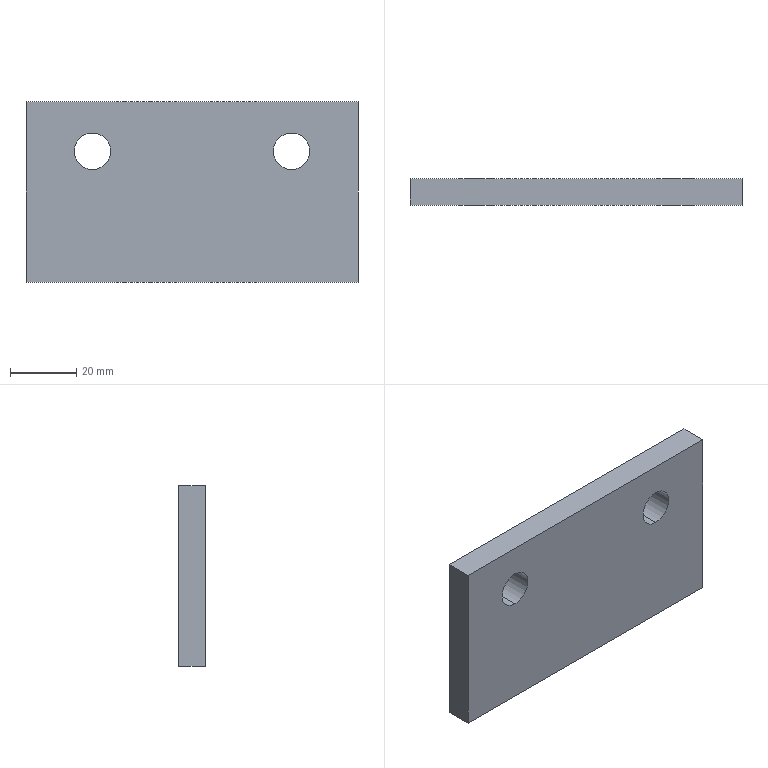Part | SolidWorks | features Extrusion 1, HoleWzd 1 | 1 solid | 10 faces | box 100 x 8 x 54.5 mm | volume 42079 mm3 | plane 6 | cylinder 4 | commonest cylinder face diameters 11 x4
STEP:
#1=CARTESIAN_POINT('',(-30.,0.,6.75));
#2=VERTEX_POINT('',#1);
#3=CARTESIAN_POINT('',(-30.,0.,17.75));
#4=VERTEX_POINT('',#3);
#5=CARTESIAN_POINT('',(-30.,0.,12.25));
#6=DIRECTION('',(0.,1.,0.));
#7=DIRECTION('',(0.,0.,1.));
#8=AXIS2_PLACEMENT_3D('',#5,#6,#7);
#9=CIRCLE('',#8,5.5);
#10=EDGE_CURVE('',#2,#4,#9,.T.);
#11=ORIENTED_EDGE('',*,*,#10,.F.);
#12=CARTESIAN_POINT('',(-30.,8.,6.75));
#13=VERTEX_POINT('',#12);
#14=CARTESIAN_POINT('',(-30.,8.,6.75));
#15=DIRECTION('',(0.,1.,0.));
#16=VECTOR('',#15,1000.);
#17=LINE('',#14,#16);
#18=EDGE_CURVE('',#2,#13,#17,.T.);
#19=ORIENTED_EDGE('',*,*,#18,.T.);
#20=CARTESIAN_POINT('',(-30.,8.,17.75));
#21=VERTEX_POINT('',#20);
#22=CARTESIAN_POINT('',(-30.,8.,12.25));
#23=DIRECTION('',(0.,1.,0.));
#24=DIRECTION('',(0.,0.,1.));
#25=AXIS2_PLACEMENT_3D('',#22,#23,#24);
#26=CIRCLE('',#25,5.5);
#27=EDGE_CURVE('',#13,#21,#26,.T.);
#28=ORIENTED_EDGE('',*,*,#27,.T.);
#29=CARTESIAN_POINT('',(-30.,8.,17.75));
#30=DIRECTION('',(0.,1.,0.));
#31=VECTOR('',#30,1000.);
#32=LINE('',#29,#31);
#33=EDGE_CURVE('',#4,#21,#32,.T.);
#34=ORIENTED_EDGE('',*,*,#33,.F.);
#35=EDGE_LOOP('',(#11,#19,#28,#34));
#36=FACE_OUTER_BOUND('',#35,.T.);
#37=CARTESIAN_POINT('',(-30.,8.,12.25));
#38=DIRECTION('',(0.,1.,0.));
#39=DIRECTION('',(0.,0.,1.));
#40=AXIS2_PLACEMENT_3D('',#37,#38,#39);
#41=CYLINDRICAL_SURFACE('',#40,5.5);
#42=ADVANCED_FACE('',(#36),#41,.F.);
#43=CARTESIAN_POINT('',(30.,0.,6.75));
#44=VERTEX_POINT('',#43);
#45=CARTESIAN_POINT('',(30.,0.,17.75));
#46=VERTEX_POINT('',#45);
#47=CARTESIAN_POINT('',(30.,0.,12.25));
#48=DIRECTION('',(0.,1.,0.));
#49=DIRECTION('',(0.,0.,1.));
#50=AXIS2_PLACEMENT_3D('',#47,#48,#49);
#51=CIRCLE('',#50,5.5);
#52=EDGE_CURVE('',#44,#46,#51,.T.);
#53=ORIENTED_EDGE('',*,*,#52,.F.);
#54=CARTESIAN_POINT('',(30.,8.,6.75));
#55=VERTEX_POINT('',#54);
#56=CARTESIAN_POINT('',(30.,8.,6.75));
#57=DIRECTION('',(0.,1.,0.));
#58=VECTOR('',#57,1000.);
#59=LINE('',#56,#58);
#60=EDGE_CURVE('',#44,#55,#59,.T.);
#61=ORIENTED_EDGE('',*,*,#60,.T.);
#62=CARTESIAN_POINT('',(30.,8.,17.75));
#63=VERTEX_POINT('',#62);
#64=CARTESIAN_POINT('',(30.,8.,12.25));
#65=DIRECTION('',(0.,1.,0.));
#66=DIRECTION('',(0.,0.,1.));
#67=AXIS2_PLACEMENT_3D('',#64,#65,#66);
#68=CIRCLE('',#67,5.5);
#69=EDGE_CURVE('',#55,#63,#68,.T.);
#70=ORIENTED_EDGE('',*,*,#69,.T.);
#71=CARTESIAN_POINT('',(30.,8.,17.75));
#72=DIRECTION('',(0.,1.,0.));
#73=VECTOR('',#72,1000.);
#74=LINE('',#71,#73);
#75=EDGE_CURVE('',#46,#63,#74,.T.);
#76=ORIENTED_EDGE('',*,*,#75,.F.);
#77=EDGE_LOOP('',(#53,#61,#70,#76));
#78=FACE_OUTER_BOUND('',#77,.T.);
#79=CARTESIAN_POINT('',(30.,8.,12.25));
#80=DIRECTION('',(0.,1.,0.));
#81=DIRECTION('',(0.,0.,1.));
#82=AXIS2_PLACEMENT_3D('',#79,#80,#81);
#83=CYLINDRICAL_SURFACE('',#82,5.5);
#84=ADVANCED_FACE('',(#78),#83,.F.);
#85=CARTESIAN_POINT('',(-50.,0.,-27.25));
#86=VERTEX_POINT('',#85);
#87=CARTESIAN_POINT('',(-50.,0.,27.25));
#88=VERTEX_POINT('',#87);
#89=CARTESIAN_POINT('',(-50.,0.,27.25));
#90=DIRECTION('',(0.,0.,1.));
#91=VECTOR('',#90,1000.);
#92=LINE('',#89,#91);
#93=EDGE_CURVE('',#86,#88,#92,.T.);
#94=ORIENTED_EDGE('',*,*,#93,.T.);
#95=CARTESIAN_POINT('',(-50.,8.,27.25));
#96=VERTEX_POINT('',#95);
#97=CARTESIAN_POINT('',(-50.,8.,27.25));
#98=DIRECTION('',(0.,-1.,0.));
#99=VECTOR('',#98,1000.);
#100=LINE('',#97,#99);
#101=EDGE_CURVE('',#96,#88,#100,.T.);
#102=ORIENTED_EDGE('',*,*,#101,.F.);
#103=CARTESIAN_POINT('',(-50.,8.,-27.25));
#104=VERTEX_POINT('',#103);
#105=CARTESIAN_POINT('',(-50.,8.,27.25));
#106=DIRECTION('',(0.,0.,1.));
#107=VECTOR('',#106,1000.);
#108=LINE('',#105,#107);
#109=EDGE_CURVE('',#104,#96,#108,.T.);
#110=ORIENTED_EDGE('',*,*,#109,.F.);
#111=CARTESIAN_POINT('',(-50.,8.,-27.25));
#112=DIRECTION('',(0.,-1.,0.));
#113=VECTOR('',#112,1000.);
#114=LINE('',#111,#113);
#115=EDGE_CURVE('',#104,#86,#114,.T.);
#116=ORIENTED_EDGE('',*,*,#115,.T.);
#117=EDGE_LOOP('',(#94,#102,#110,#116));
#118=FACE_OUTER_BOUND('',#117,.T.);
#119=CARTESIAN_POINT('',(-50.,8.,27.25));
#120=DIRECTION('',(1.,0.,0.));
#121=DIRECTION('',(0.,0.,-1.));
#122=AXIS2_PLACEMENT_3D('',#119,#120,#121);
#123=PLANE('',#122);
#124=ADVANCED_FACE('',(#118),#123,.F.);
#125=CARTESIAN_POINT('',(50.,0.,27.25));
#126=VERTEX_POINT('',#125);
#127=CARTESIAN_POINT('',(50.,0.,27.25));
#128=DIRECTION('',(1.,0.,0.));
#129=VECTOR('',#128,1000.);
#130=LINE('',#127,#129);
#131=EDGE_CURVE('',#88,#126,#130,.T.);
#132=ORIENTED_EDGE('',*,*,#131,.T.);
#133=CARTESIAN_POINT('',(50.,8.,27.25));
#134=VERTEX_POINT('',#133);
#135=CARTESIAN_POINT('',(50.,8.,27.25));
#136=DIRECTION('',(0.,-1.,0.));
#137=VECTOR('',#136,1000.);
#138=LINE('',#135,#137);
#139=EDGE_CURVE('',#134,#126,#138,.T.);
#140=ORIENTED_EDGE('',*,*,#139,.F.);
#141=CARTESIAN_POINT('',(50.,8.,27.25));
#142=DIRECTION('',(1.,0.,0.));
#143=VECTOR('',#142,1000.);
#144=LINE('',#141,#143);
#145=EDGE_CURVE('',#96,#134,#144,.T.);
#146=ORIENTED_EDGE('',*,*,#145,.F.);
#147=ORIENTED_EDGE('',*,*,#101,.T.);
#148=EDGE_LOOP('',(#132,#140,#146,#147));
#149=FACE_OUTER_BOUND('',#148,.T.);
#150=CARTESIAN_POINT('',(50.,8.,27.25));
#151=DIRECTION('',(0.,0.,-1.));
#152=DIRECTION('',(-1.,0.,0.));
#153=AXIS2_PLACEMENT_3D('',#150,#151,#152);
#154=PLANE('',#153);
#155=ADVANCED_FACE('',(#149),#154,.F.);
#156=CARTESIAN_POINT('',(50.,0.,-27.25));
#157=VERTEX_POINT('',#156);
#158=CARTESIAN_POINT('',(50.,0.,27.25));
#159=DIRECTION('',(0.,0.,-1.));
#160=VECTOR('',#159,1000.);
#161=LINE('',#158,#160);
#162=EDGE_CURVE('',#126,#157,#161,.T.);
#163=ORIENTED_EDGE('',*,*,#162,.T.);
#164=CARTESIAN_POINT('',(50.,8.,-27.25));
#165=VERTEX_POINT('',#164);
#166=CARTESIAN_POINT('',(50.,8.,-27.25));
#167=DIRECTION('',(0.,-1.,0.));
#168=VECTOR('',#167,1000.);
#169=LINE('',#166,#168);
#170=EDGE_CURVE('',#165,#157,#169,.T.);
#171=ORIENTED_EDGE('',*,*,#170,.F.);
#172=CARTESIAN_POINT('',(50.,8.,27.25));
#173=DIRECTION('',(0.,0.,-1.));
#174=VECTOR('',#173,1000.);
#175=LINE('',#172,#174);
#176=EDGE_CURVE('',#134,#165,#175,.T.);
#177=ORIENTED_EDGE('',*,*,#176,.F.);
#178=ORIENTED_EDGE('',*,*,#139,.T.);
#179=EDGE_LOOP('',(#163,#171,#177,#178));
#180=FACE_OUTER_BOUND('',#179,.T.);
#181=CARTESIAN_POINT('',(50.,8.,27.25));
#182=DIRECTION('',(-1.,0.,0.));
#183=DIRECTION('',(0.,0.,1.));
#184=AXIS2_PLACEMENT_3D('',#181,#182,#183);
#185=PLANE('',#184);
#186=ADVANCED_FACE('',(#180),#185,.F.);
#187=CARTESIAN_POINT('',(50.,0.,-27.25));
#188=DIRECTION('',(-1.,0.,0.));
#189=VECTOR('',#188,1000.);
#190=LINE('',#187,#189);
#191=EDGE_CURVE('',#157,#86,#190,.T.);
#192=ORIENTED_EDGE('',*,*,#191,.T.);
#193=ORIENTED_EDGE('',*,*,#115,.F.);
#194=CARTESIAN_POINT('',(50.,8.,-27.25));
#195=DIRECTION('',(-1.,0.,0.));
#196=VECTOR('',#195,1000.);
#197=LINE('',#194,#196);
#198=EDGE_CURVE('',#165,#104,#197,.T.);
#199=ORIENTED_EDGE('',*,*,#198,.F.);
#200=ORIENTED_EDGE('',*,*,#170,.T.);
#201=EDGE_LOOP('',(#192,#193,#199,#200));
#202=FACE_OUTER_BOUND('',#201,.T.);
#203=CARTESIAN_POINT('',(50.,8.,-27.25));
#204=DIRECTION('',(0.,0.,1.));
#205=DIRECTION('',(1.,0.,0.));
#206=AXIS2_PLACEMENT_3D('',#203,#204,#205);
#207=PLANE('',#206);
#208=ADVANCED_FACE('',(#202),#207,.F.);
#209=CARTESIAN_POINT('',(-30.,8.,12.25));
#210=DIRECTION('',(0.,1.,0.));
#211=DIRECTION('',(0.,0.,1.));
#212=AXIS2_PLACEMENT_3D('',#209,#210,#211);
#213=CIRCLE('',#212,5.5);
#214=EDGE_CURVE('',#21,#13,#213,.T.);
#215=ORIENTED_EDGE('',*,*,#214,.F.);
#216=ORIENTED_EDGE('',*,*,#27,.F.);
#217=EDGE_LOOP('',(#215,#216));
#218=FACE_BOUND('',#217,.T.);
#219=CARTESIAN_POINT('',(30.,8.,12.25));
#220=DIRECTION('',(0.,1.,0.));
#221=DIRECTION('',(0.,0.,1.));
#222=AXIS2_PLACEMENT_3D('',#219,#220,#221);
#223=CIRCLE('',#222,5.5);
#224=EDGE_CURVE('',#63,#55,#223,.T.);
#225=ORIENTED_EDGE('',*,*,#224,.F.);
#226=ORIENTED_EDGE('',*,*,#69,.F.);
#227=EDGE_LOOP('',(#225,#226));
#228=FACE_BOUND('',#227,.T.);
#229=ORIENTED_EDGE('',*,*,#109,.T.);
#230=ORIENTED_EDGE('',*,*,#145,.T.);
#231=ORIENTED_EDGE('',*,*,#176,.T.);
#232=ORIENTED_EDGE('',*,*,#198,.T.);
#233=EDGE_LOOP('',(#229,#230,#231,#232));
#234=FACE_OUTER_BOUND('',#233,.T.);
#235=CARTESIAN_POINT('',(0.,8.,0.));
#236=DIRECTION('',(0.,1.,0.));
#237=DIRECTION('',(0.,0.,1.));
#238=AXIS2_PLACEMENT_3D('',#235,#236,#237);
#239=PLANE('',#238);
#240=ADVANCED_FACE('',(#218,#228,#234),#239,.T.);
#241=CARTESIAN_POINT('',(-30.,0.,12.25));
#242=DIRECTION('',(0.,1.,0.));
#243=DIRECTION('',(0.,0.,1.));
#244=AXIS2_PLACEMENT_3D('',#241,#242,#243);
#245=CIRCLE('',#244,5.5);
#246=EDGE_CURVE('',#4,#2,#245,.T.);
#247=ORIENTED_EDGE('',*,*,#246,.T.);
#248=ORIENTED_EDGE('',*,*,#10,.T.);
#249=EDGE_LOOP('',(#247,#248));
#250=FACE_BOUND('',#249,.T.);
#251=CARTESIAN_POINT('',(30.,0.,12.25));
#252=DIRECTION('',(0.,1.,0.));
#253=DIRECTION('',(0.,0.,1.));
#254=AXIS2_PLACEMENT_3D('',#251,#252,#253);
#255=CIRCLE('',#254,5.5);
#256=EDGE_CURVE('',#46,#44,#255,.T.);
#257=ORIENTED_EDGE('',*,*,#256,.T.);
#258=ORIENTED_EDGE('',*,*,#52,.T.);
#259=EDGE_LOOP('',(#257,#258));
#260=FACE_BOUND('',#259,.T.);
#261=ORIENTED_EDGE('',*,*,#93,.F.);
#262=ORIENTED_EDGE('',*,*,#191,.F.);
#263=ORIENTED_EDGE('',*,*,#162,.F.);
#264=ORIENTED_EDGE('',*,*,#131,.F.);
#265=EDGE_LOOP('',(#261,#262,#263,#264));
#266=FACE_OUTER_BOUND('',#265,.T.);
#267=CARTESIAN_POINT('',(0.,0.,0.));
#268=DIRECTION('',(0.,1.,0.));
#269=DIRECTION('',(0.,0.,1.));
#270=AXIS2_PLACEMENT_3D('',#267,#268,#269);
#271=PLANE('',#270);
#272=ADVANCED_FACE('',(#250,#260,#266),#271,.F.);
#273=ORIENTED_EDGE('',*,*,#60,.F.);
#274=ORIENTED_EDGE('',*,*,#256,.F.);
#275=ORIENTED_EDGE('',*,*,#75,.T.);
#276=ORIENTED_EDGE('',*,*,#224,.T.);
#277=EDGE_LOOP('',(#273,#274,#275,#276));
#278=FACE_OUTER_BOUND('',#277,.T.);
#279=CARTESIAN_POINT('',(30.,8.,12.25));
#280=DIRECTION('',(0.,1.,0.));
#281=DIRECTION('',(0.,0.,1.));
#282=AXIS2_PLACEMENT_3D('',#279,#280,#281);
#283=CYLINDRICAL_SURFACE('',#282,5.5);
#284=ADVANCED_FACE('',(#278),#283,.F.);
#285=ORIENTED_EDGE('',*,*,#18,.F.);
#286=ORIENTED_EDGE('',*,*,#246,.F.);
#287=ORIENTED_EDGE('',*,*,#33,.T.);
#288=ORIENTED_EDGE('',*,*,#214,.T.);
#289=EDGE_LOOP('',(#285,#286,#287,#288));
#290=FACE_OUTER_BOUND('',#289,.T.);
#291=CARTESIAN_POINT('',(-30.,8.,12.25));
#292=DIRECTION('',(0.,1.,0.));
#293=DIRECTION('',(0.,0.,1.));
#294=AXIS2_PLACEMENT_3D('',#291,#292,#293);
#295=CYLINDRICAL_SURFACE('',#294,5.5);
#296=ADVANCED_FACE('',(#290),#295,.F.);
#297=CLOSED_SHELL('',(#42,#84,#124,#155,#186,#208,#240,#272,#284,#296));
#298=MANIFOLD_SOLID_BREP('',#297);
#299=CARTESIAN_POINT('',(0.,0.,0.));
#300=DIRECTION('',(0.,0.,1.));
#301=DIRECTION('',(1.,0.,0.));
#302=AXIS2_PLACEMENT_3D('',#299,#300,#301);
#303=(LENGTH_UNIT()NAMED_UNIT(*)SI_UNIT(.MILLI.,.METRE.));
#304=UNCERTAINTY_MEASURE_WITH_UNIT(LENGTH_MEASURE(0.00001),#303,'','');
#305=(NAMED_UNIT(*)PLANE_ANGLE_UNIT()SI_UNIT($,.RADIAN.));
#306=(NAMED_UNIT(*)SI_UNIT($,.STERADIAN.)SOLID_ANGLE_UNIT());
#307=(GEOMETRIC_REPRESENTATION_CONTEXT(3)GLOBAL_UNCERTAINTY_ASSIGNED_CONTEXT((#304))GLOBAL_UNIT_ASSIGNED_CONTEXT((#303,#305,#306))REPRESENTATION_CONTEXT('',''));
#308=ADVANCED_BREP_SHAPE_REPRESENTATION('',(#298,#302),#307);